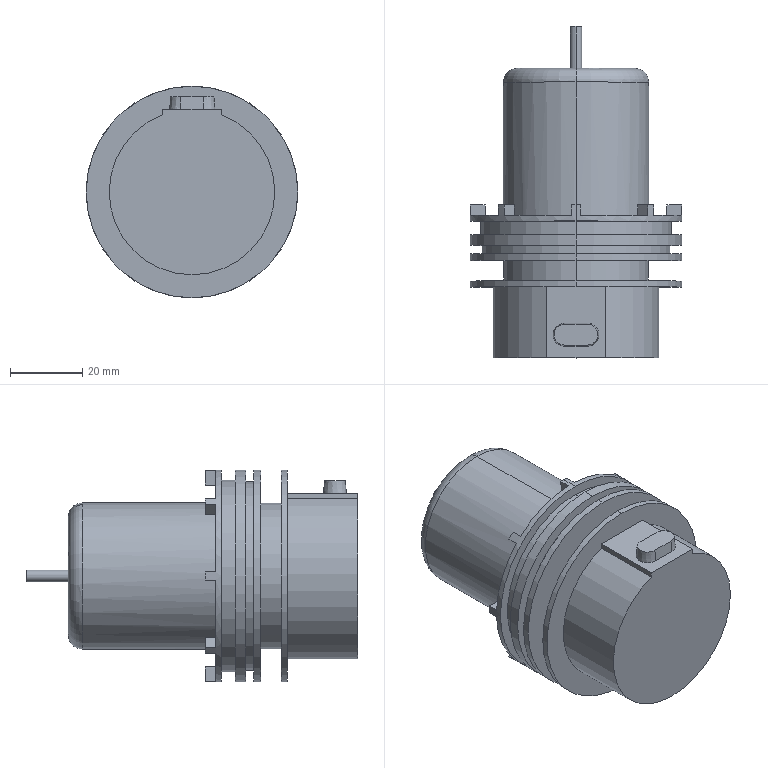Part | SolidWorks | features ICE 14, Fillet 2, CirPattern 1, Cut 1, Extrusion 1, RefAxis 1, RevCut 1 | 1 solid | 122 faces | box 58.42 x 91.643 x 58.42 mm | volume 118735 mm3 | plane 73 | cylinder 24 | cone 19 | torus 6 | commonest cylinder face diameters 58.42 x8 3.175 x2 6.985 x2 40.132 x2 40.335 x2 45.72 x2